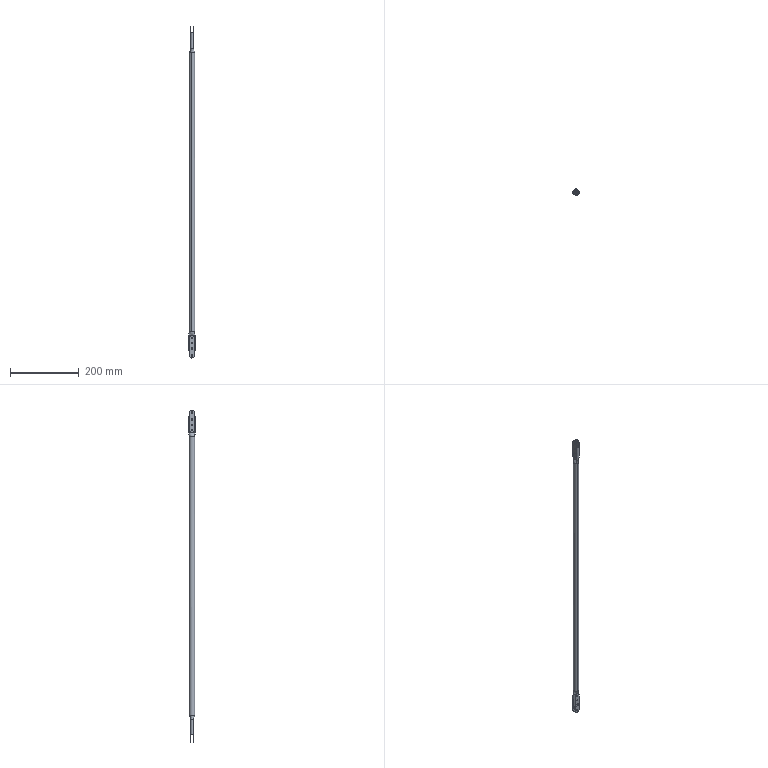Part | SolidWorks | features BaseBody 2 | 2 solids | 101 faces | box 19.559 x 19.559 x 962.5 mm | volume 44204 mm3 | cylinder 53 | plane 36 | spline 12 | commonest cylinder face diameters 3.175 x24 15 x12 4.826 x8 6.858 x5 14.097 x2 15.875 x2